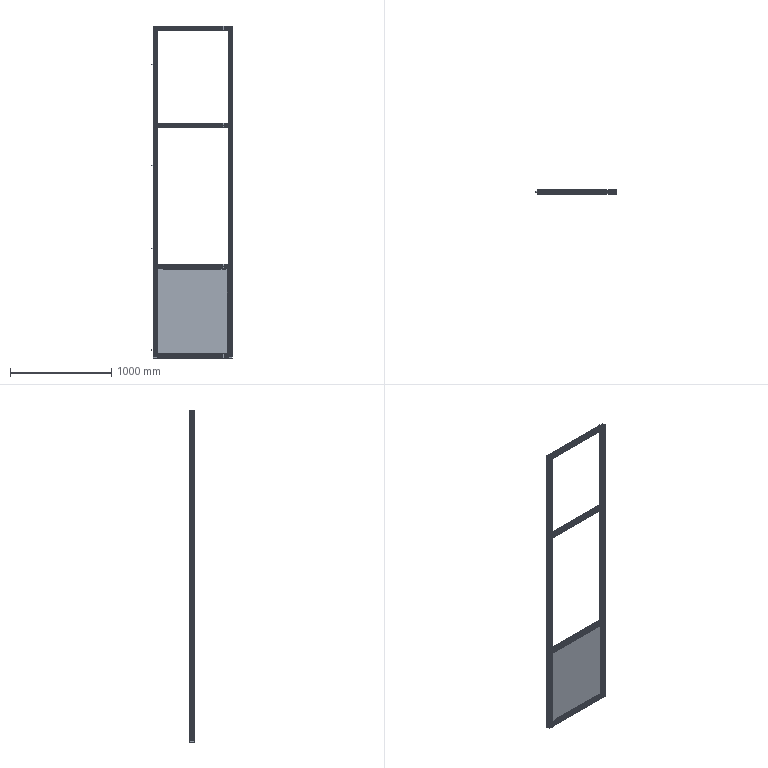Part | SolidWorks | features ReferencePattern 12, LocalLPattern 3 | 23 solids | 1946 faces | box 792.4 x 40 x 3280 mm | volume 8824321 mm3 | plane 1348 | cylinder 546 | cone 44 | spline 8 | commonest cylinder face diameters 6.8 x142 2 x68 19 x48 1 x36 6.6 x32 11 x32